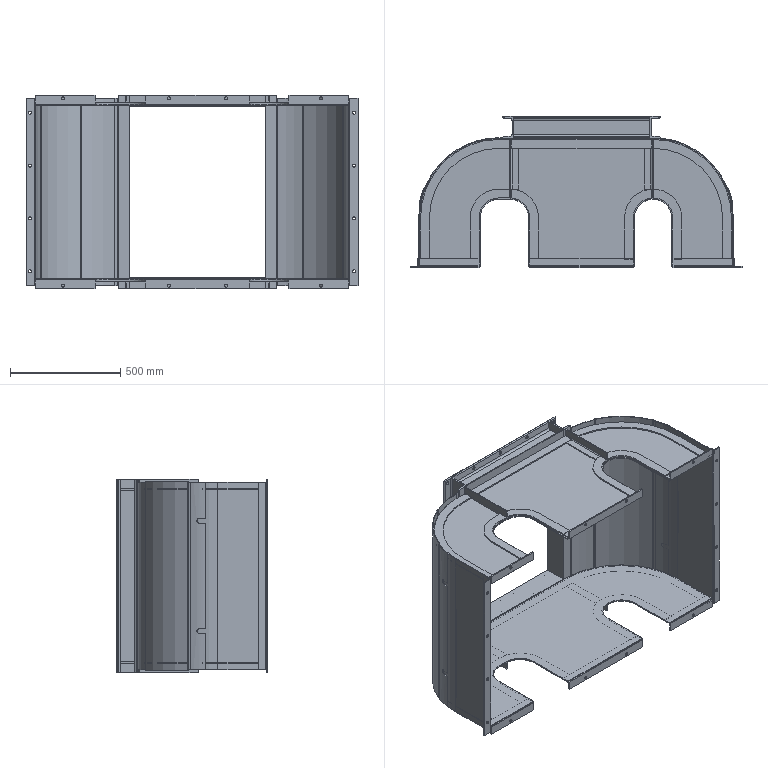Part | NX | features BREP 16, DATUM_CSYS 2, SKETCH 2 | 30 solids | 426 faces | box 1506 x 685 x 876 mm | volume 16741926 mm3 | plane 284 | cylinder 142 | commonest cylinder face diameters 14 x64 10 x12 720 x10 8.4 x8 17 x8 726 x8